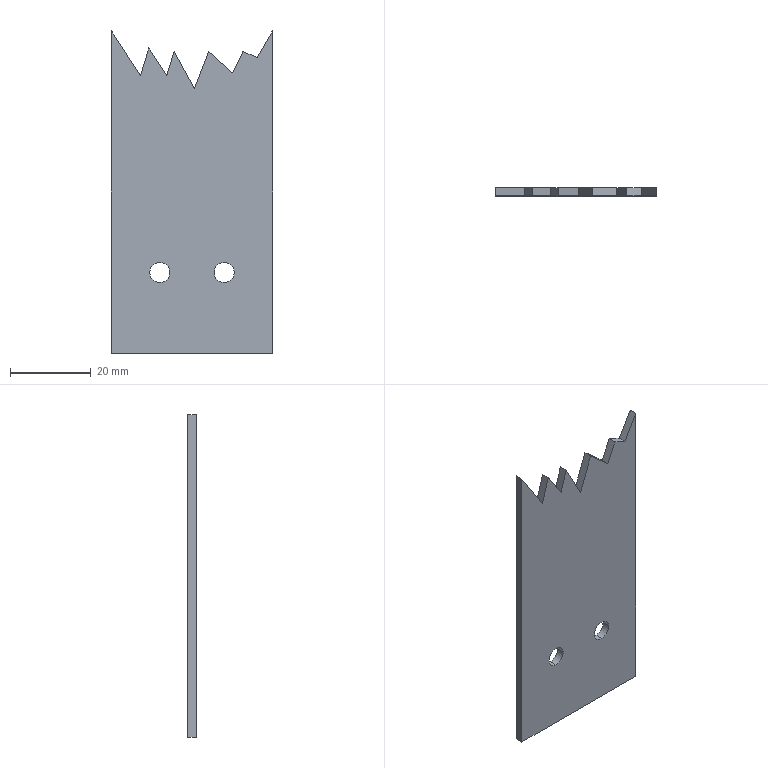Part | SolidWorks | features Cut 2, Extrusion 1 | 1 solid | 19 faces | box 40 x 2 x 80 mm | volume 5747 mm3 | plane 15 | cylinder 4 | commonest cylinder face diameters 5 x4
STEP:
#1=CARTESIAN_POINT('',(8.,2.,-22.5));
#2=VERTEX_POINT('',#1);
#3=CARTESIAN_POINT('',(8.,2.,-17.5));
#4=VERTEX_POINT('',#3);
#5=CARTESIAN_POINT('',(8.,2.,-20.));
#6=DIRECTION('',(0.,1.,0.));
#7=DIRECTION('',(0.,0.,1.));
#8=AXIS2_PLACEMENT_3D('',#5,#6,#7);
#9=CIRCLE('',#8,2.5);
#10=EDGE_CURVE('',#2,#4,#9,.T.);
#11=ORIENTED_EDGE('',*,*,#10,.T.);
#12=CARTESIAN_POINT('',(8.,0.,-17.5));
#13=VERTEX_POINT('',#12);
#14=CARTESIAN_POINT('',(8.,10.,-17.5));
#15=DIRECTION('',(0.,-1.,0.));
#16=VECTOR('',#15,1000.);
#17=LINE('',#14,#16);
#18=EDGE_CURVE('',#4,#13,#17,.T.);
#19=ORIENTED_EDGE('',*,*,#18,.T.);
#20=CARTESIAN_POINT('',(8.,0.,-22.5));
#21=VERTEX_POINT('',#20);
#22=CARTESIAN_POINT('',(8.,0.,-20.));
#23=DIRECTION('',(0.,-1.,0.));
#24=DIRECTION('',(0.,0.,-1.));
#25=AXIS2_PLACEMENT_3D('',#22,#23,#24);
#26=CIRCLE('',#25,2.5);
#27=EDGE_CURVE('',#13,#21,#26,.T.);
#28=ORIENTED_EDGE('',*,*,#27,.T.);
#29=CARTESIAN_POINT('',(8.,10.,-22.5));
#30=DIRECTION('',(0.,-1.,0.));
#31=VECTOR('',#30,1000.);
#32=LINE('',#29,#31);
#33=EDGE_CURVE('',#2,#21,#32,.T.);
#34=ORIENTED_EDGE('',*,*,#33,.F.);
#35=EDGE_LOOP('',(#11,#19,#28,#34));
#36=FACE_OUTER_BOUND('',#35,.T.);
#37=CARTESIAN_POINT('',(8.,10.,-20.));
#38=DIRECTION('',(0.,-1.,0.));
#39=DIRECTION('',(0.,0.,-1.));
#40=AXIS2_PLACEMENT_3D('',#37,#38,#39);
#41=CYLINDRICAL_SURFACE('',#40,2.5);
#42=ADVANCED_FACE('',(#36),#41,.F.);
#43=CARTESIAN_POINT('',(-8.,2.,-22.5));
#44=VERTEX_POINT('',#43);
#45=CARTESIAN_POINT('',(-8.,2.,-17.5));
#46=VERTEX_POINT('',#45);
#47=CARTESIAN_POINT('',(-8.,2.,-20.));
#48=DIRECTION('',(0.,1.,0.));
#49=DIRECTION('',(0.,0.,1.));
#50=AXIS2_PLACEMENT_3D('',#47,#48,#49);
#51=CIRCLE('',#50,2.5);
#52=EDGE_CURVE('',#44,#46,#51,.T.);
#53=ORIENTED_EDGE('',*,*,#52,.T.);
#54=CARTESIAN_POINT('',(-8.,0.,-17.5));
#55=VERTEX_POINT('',#54);
#56=CARTESIAN_POINT('',(-8.,10.,-17.5));
#57=DIRECTION('',(0.,-1.,0.));
#58=VECTOR('',#57,1000.);
#59=LINE('',#56,#58);
#60=EDGE_CURVE('',#46,#55,#59,.T.);
#61=ORIENTED_EDGE('',*,*,#60,.T.);
#62=CARTESIAN_POINT('',(-8.,0.,-22.5));
#63=VERTEX_POINT('',#62);
#64=CARTESIAN_POINT('',(-8.,0.,-20.));
#65=DIRECTION('',(0.,-1.,0.));
#66=DIRECTION('',(0.,0.,-1.));
#67=AXIS2_PLACEMENT_3D('',#64,#65,#66);
#68=CIRCLE('',#67,2.5);
#69=EDGE_CURVE('',#55,#63,#68,.T.);
#70=ORIENTED_EDGE('',*,*,#69,.T.);
#71=CARTESIAN_POINT('',(-8.,10.,-22.5));
#72=DIRECTION('',(0.,-1.,0.));
#73=VECTOR('',#72,1000.);
#74=LINE('',#71,#73);
#75=EDGE_CURVE('',#44,#63,#74,.T.);
#76=ORIENTED_EDGE('',*,*,#75,.F.);
#77=EDGE_LOOP('',(#53,#61,#70,#76));
#78=FACE_OUTER_BOUND('',#77,.T.);
#79=CARTESIAN_POINT('',(-8.,10.,-20.));
#80=DIRECTION('',(0.,-1.,0.));
#81=DIRECTION('',(0.,0.,-1.));
#82=AXIS2_PLACEMENT_3D('',#79,#80,#81);
#83=CYLINDRICAL_SURFACE('',#82,2.5);
#84=ADVANCED_FACE('',(#78),#83,.F.);
#85=CARTESIAN_POINT('',(20.,0.,40.));
#86=VERTEX_POINT('',#85);
#87=CARTESIAN_POINT('',(20.,0.,-40.));
#88=VERTEX_POINT('',#87);
#89=CARTESIAN_POINT('',(20.,0.,-40.));
#90=DIRECTION('',(0.,0.,-1.));
#91=VECTOR('',#90,1000.);
#92=LINE('',#89,#91);
#93=EDGE_CURVE('',#86,#88,#92,.T.);
#94=ORIENTED_EDGE('',*,*,#93,.T.);
#95=CARTESIAN_POINT('',(20.,2.,-40.));
#96=VERTEX_POINT('',#95);
#97=CARTESIAN_POINT('',(20.,2.,-40.));
#98=DIRECTION('',(0.,-1.,0.));
#99=VECTOR('',#98,1000.);
#100=LINE('',#97,#99);
#101=EDGE_CURVE('',#96,#88,#100,.T.);
#102=ORIENTED_EDGE('',*,*,#101,.F.);
#103=CARTESIAN_POINT('',(20.,2.,40.));
#104=VERTEX_POINT('',#103);
#105=CARTESIAN_POINT('',(20.,2.,-40.));
#106=DIRECTION('',(0.,0.,-1.));
#107=VECTOR('',#106,1000.);
#108=LINE('',#105,#107);
#109=EDGE_CURVE('',#104,#96,#108,.T.);
#110=ORIENTED_EDGE('',*,*,#109,.F.);
#111=CARTESIAN_POINT('',(20.,2.,40.));
#112=DIRECTION('',(0.,-1.,0.));
#113=VECTOR('',#112,1000.);
#114=LINE('',#111,#113);
#115=EDGE_CURVE('',#104,#86,#114,.T.);
#116=ORIENTED_EDGE('',*,*,#115,.T.);
#117=EDGE_LOOP('',(#94,#102,#110,#116));
#118=FACE_OUTER_BOUND('',#117,.T.);
#119=CARTESIAN_POINT('',(20.,2.,-40.));
#120=DIRECTION('',(-1.,0.,0.));
#121=DIRECTION('',(0.,0.,1.));
#122=AXIS2_PLACEMENT_3D('',#119,#120,#121);
#123=PLANE('',#122);
#124=ADVANCED_FACE('',(#118),#123,.F.);
#125=CARTESIAN_POINT('',(-20.,0.,-40.));
#126=VERTEX_POINT('',#125);
#127=CARTESIAN_POINT('',(-20.,0.,-40.));
#128=DIRECTION('',(-1.,0.,0.));
#129=VECTOR('',#128,1000.);
#130=LINE('',#127,#129);
#131=EDGE_CURVE('',#88,#126,#130,.T.);
#132=ORIENTED_EDGE('',*,*,#131,.T.);
#133=CARTESIAN_POINT('',(-20.,2.,-40.));
#134=VERTEX_POINT('',#133);
#135=CARTESIAN_POINT('',(-20.,2.,-40.));
#136=DIRECTION('',(0.,-1.,0.));
#137=VECTOR('',#136,1000.);
#138=LINE('',#135,#137);
#139=EDGE_CURVE('',#134,#126,#138,.T.);
#140=ORIENTED_EDGE('',*,*,#139,.F.);
#141=CARTESIAN_POINT('',(-20.,2.,-40.));
#142=DIRECTION('',(-1.,0.,0.));
#143=VECTOR('',#142,1000.);
#144=LINE('',#141,#143);
#145=EDGE_CURVE('',#96,#134,#144,.T.);
#146=ORIENTED_EDGE('',*,*,#145,.F.);
#147=ORIENTED_EDGE('',*,*,#101,.T.);
#148=EDGE_LOOP('',(#132,#140,#146,#147));
#149=FACE_OUTER_BOUND('',#148,.T.);
#150=CARTESIAN_POINT('',(-20.,2.,-40.));
#151=DIRECTION('',(0.,0.,1.));
#152=DIRECTION('',(1.,0.,0.));
#153=AXIS2_PLACEMENT_3D('',#150,#151,#152);
#154=PLANE('',#153);
#155=ADVANCED_FACE('',(#149),#154,.F.);
#156=CARTESIAN_POINT('',(-20.,0.,40.));
#157=VERTEX_POINT('',#156);
#158=CARTESIAN_POINT('',(-20.,0.,-40.));
#159=DIRECTION('',(0.,0.,1.));
#160=VECTOR('',#159,1000.);
#161=LINE('',#158,#160);
#162=EDGE_CURVE('',#126,#157,#161,.T.);
#163=ORIENTED_EDGE('',*,*,#162,.T.);
#164=CARTESIAN_POINT('',(-20.,2.,40.));
#165=VERTEX_POINT('',#164);
#166=CARTESIAN_POINT('',(-20.,2.,40.));
#167=DIRECTION('',(0.,-1.,0.));
#168=VECTOR('',#167,1000.);
#169=LINE('',#166,#168);
#170=EDGE_CURVE('',#165,#157,#169,.T.);
#171=ORIENTED_EDGE('',*,*,#170,.F.);
#172=CARTESIAN_POINT('',(-20.,2.,-40.));
#173=DIRECTION('',(0.,0.,1.));
#174=VECTOR('',#173,1000.);
#175=LINE('',#172,#174);
#176=EDGE_CURVE('',#134,#165,#175,.T.);
#177=ORIENTED_EDGE('',*,*,#176,.F.);
#178=ORIENTED_EDGE('',*,*,#139,.T.);
#179=EDGE_LOOP('',(#163,#171,#177,#178));
#180=FACE_OUTER_BOUND('',#179,.T.);
#181=CARTESIAN_POINT('',(-20.,2.,-40.));
#182=DIRECTION('',(1.,0.,0.));
#183=DIRECTION('',(0.,0.,-1.));
#184=AXIS2_PLACEMENT_3D('',#181,#182,#183);
#185=PLANE('',#184);
#186=ADVANCED_FACE('',(#180),#185,.F.);
#187=CARTESIAN_POINT('',(-12.785,2.,28.891));
#188=VERTEX_POINT('',#187);
#189=CARTESIAN_POINT('',(-20.,2.,40.));
#190=DIRECTION('',(-0.5447,0.,0.8386));
#191=VECTOR('',#190,1000.);
#192=LINE('',#189,#191);
#193=EDGE_CURVE('',#188,#165,#192,.T.);
#194=ORIENTED_EDGE('',*,*,#193,.F.);
#195=CARTESIAN_POINT('',(-10.737,2.,35.779));
#196=VERTEX_POINT('',#195);
#197=CARTESIAN_POINT('',(-12.785,2.,28.891));
#198=DIRECTION('',(-0.285,0.,-0.9585));
#199=VECTOR('',#198,1000.);
#200=LINE('',#197,#199);
#201=EDGE_CURVE('',#196,#188,#200,.T.);
#202=ORIENTED_EDGE('',*,*,#201,.F.);
#203=CARTESIAN_POINT('',(-6.263,2.,28.891));
#204=VERTEX_POINT('',#203);
#205=CARTESIAN_POINT('',(-10.737,2.,35.779));
#206=DIRECTION('',(-0.5447,0.,0.8386));
#207=VECTOR('',#206,1000.);
#208=LINE('',#205,#207);
#209=EDGE_CURVE('',#204,#196,#208,.T.);
#210=ORIENTED_EDGE('',*,*,#209,.F.);
#211=CARTESIAN_POINT('',(-4.459,2.,34.96));
#212=VERTEX_POINT('',#211);
#213=CARTESIAN_POINT('',(-6.263,2.,28.891));
#214=DIRECTION('',(-0.285,0.,-0.9585));
#215=VECTOR('',#214,1000.);
#216=LINE('',#213,#215);
#217=EDGE_CURVE('',#212,#204,#216,.T.);
#218=ORIENTED_EDGE('',*,*,#217,.F.);
#219=CARTESIAN_POINT('',(0.6034,2.,25.613));
#220=VERTEX_POINT('',#219);
#221=CARTESIAN_POINT('',(-4.459,2.,34.96));
#222=DIRECTION('',(-0.4763,0.,0.8793));
#223=VECTOR('',#222,1000.);
#224=LINE('',#221,#223);
#225=EDGE_CURVE('',#220,#212,#224,.T.);
#226=ORIENTED_EDGE('',*,*,#225,.F.);
#227=CARTESIAN_POINT('',(4.155,2.,34.96));
#228=VERTEX_POINT('',#227);
#229=CARTESIAN_POINT('',(0.6034,2.,25.613));
#230=DIRECTION('',(-0.3552,0.,-0.9348));
#231=VECTOR('',#230,1000.);
#232=LINE('',#229,#231);
#233=EDGE_CURVE('',#228,#220,#232,.T.);
#234=ORIENTED_EDGE('',*,*,#233,.F.);
#235=CARTESIAN_POINT('',(10.181,2.,29.56));
#236=VERTEX_POINT('',#235);
#237=CARTESIAN_POINT('',(4.155,2.,34.96));
#238=DIRECTION('',(-0.7448,0.,0.6673));
#239=VECTOR('',#238,1000.);
#240=LINE('',#237,#239);
#241=EDGE_CURVE('',#236,#228,#240,.T.);
#242=ORIENTED_EDGE('',*,*,#241,.F.);
#243=CARTESIAN_POINT('',(12.655,2.,34.96));
#244=VERTEX_POINT('',#243);
#245=CARTESIAN_POINT('',(10.181,2.,29.56));
#246=DIRECTION('',(-0.4166,0.,-0.9091));
#247=VECTOR('',#246,1000.);
#248=LINE('',#245,#247);
#249=EDGE_CURVE('',#244,#236,#248,.T.);
#250=ORIENTED_EDGE('',*,*,#249,.F.);
#251=CARTESIAN_POINT('',(16.161,2.,33.353));
#252=VERTEX_POINT('',#251);
#253=CARTESIAN_POINT('',(12.655,2.,34.96));
#254=DIRECTION('',(-0.9091,0.,0.4166));
#255=VECTOR('',#254,1000.);
#256=LINE('',#253,#255);
#257=EDGE_CURVE('',#252,#244,#256,.T.);
#258=ORIENTED_EDGE('',*,*,#257,.F.);
#259=CARTESIAN_POINT('',(16.161,2.,33.353));
#260=DIRECTION('',(-0.5001,0.,-0.8659));
#261=VECTOR('',#260,1000.);
#262=LINE('',#259,#261);
#263=EDGE_CURVE('',#104,#252,#262,.T.);
#264=ORIENTED_EDGE('',*,*,#263,.F.);
#265=ORIENTED_EDGE('',*,*,#109,.T.);
#266=ORIENTED_EDGE('',*,*,#145,.T.);
#267=ORIENTED_EDGE('',*,*,#176,.T.);
#268=EDGE_LOOP('',(#194,#202,#210,#218,#226,#234,#242,#250,#258,#264,#265,#266,#267));
#269=FACE_OUTER_BOUND('',#268,.T.);
#270=ORIENTED_EDGE('',*,*,#10,.F.);
#271=CARTESIAN_POINT('',(8.,2.,-20.));
#272=DIRECTION('',(0.,1.,0.));
#273=DIRECTION('',(0.,0.,1.));
#274=AXIS2_PLACEMENT_3D('',#271,#272,#273);
#275=CIRCLE('',#274,2.5);
#276=EDGE_CURVE('',#4,#2,#275,.T.);
#277=ORIENTED_EDGE('',*,*,#276,.F.);
#278=EDGE_LOOP('',(#270,#277));
#279=FACE_BOUND('',#278,.T.);
#280=ORIENTED_EDGE('',*,*,#52,.F.);
#281=CARTESIAN_POINT('',(-8.,2.,-20.));
#282=DIRECTION('',(0.,1.,0.));
#283=DIRECTION('',(0.,0.,1.));
#284=AXIS2_PLACEMENT_3D('',#281,#282,#283);
#285=CIRCLE('',#284,2.5);
#286=EDGE_CURVE('',#46,#44,#285,.T.);
#287=ORIENTED_EDGE('',*,*,#286,.F.);
#288=EDGE_LOOP('',(#280,#287));
#289=FACE_BOUND('',#288,.T.);
#290=CARTESIAN_POINT('',(0.,2.,0.));
#291=DIRECTION('',(0.,1.,0.));
#292=DIRECTION('',(0.,0.,1.));
#293=AXIS2_PLACEMENT_3D('',#290,#291,#292);
#294=PLANE('',#293);
#295=ADVANCED_FACE('',(#269,#279,#289),#294,.T.);
#296=CARTESIAN_POINT('',(8.,0.,-20.));
#297=DIRECTION('',(0.,-1.,0.));
#298=DIRECTION('',(0.,0.,-1.));
#299=AXIS2_PLACEMENT_3D('',#296,#297,#298);
#300=CIRCLE('',#299,2.5);
#301=EDGE_CURVE('',#21,#13,#300,.T.);
#302=ORIENTED_EDGE('',*,*,#301,.F.);
#303=ORIENTED_EDGE('',*,*,#27,.F.);
#304=EDGE_LOOP('',(#302,#303));
#305=FACE_BOUND('',#304,.T.);
#306=CARTESIAN_POINT('',(-8.,0.,-20.));
#307=DIRECTION('',(0.,-1.,0.));
#308=DIRECTION('',(0.,0.,-1.));
#309=AXIS2_PLACEMENT_3D('',#306,#307,#308);
#310=CIRCLE('',#309,2.5);
#311=EDGE_CURVE('',#63,#55,#310,.T.);
#312=ORIENTED_EDGE('',*,*,#311,.F.);
#313=ORIENTED_EDGE('',*,*,#69,.F.);
#314=EDGE_LOOP('',(#312,#313));
#315=FACE_BOUND('',#314,.T.);
#316=CARTESIAN_POINT('',(-10.737,0.,35.779));
#317=VERTEX_POINT('',#316);
#318=CARTESIAN_POINT('',(-12.785,0.,28.891));
#319=VERTEX_POINT('',#318);
#320=CARTESIAN_POINT('',(-19.638,0.,5.838));
#321=DIRECTION('',(-0.285,0.,-0.9585));
#322=VECTOR('',#321,1000.);
#323=LINE('',#320,#322);
#324=EDGE_CURVE('',#317,#319,#323,.T.);
#325=ORIENTED_EDGE('',*,*,#324,.T.);
#326=CARTESIAN_POINT('',(4.206,0.,2.732));
#327=DIRECTION('',(-0.5447,0.,0.8386));
#328=VECTOR('',#327,1000.);
#329=LINE('',#326,#328);
#330=EDGE_CURVE('',#319,#157,#329,.T.);
#331=ORIENTED_EDGE('',*,*,#330,.T.);
#332=ORIENTED_EDGE('',*,*,#162,.F.);
#333=ORIENTED_EDGE('',*,*,#131,.F.);
#334=ORIENTED_EDGE('',*,*,#93,.F.);
#335=CARTESIAN_POINT('',(16.161,0.,33.353));
#336=VERTEX_POINT('',#335);
#337=CARTESIAN_POINT('',(-2.326,0.,1.344));
#338=DIRECTION('',(-0.5001,0.,-0.8659));
#339=VECTOR('',#338,1000.);
#340=LINE('',#337,#339);
#341=EDGE_CURVE('',#86,#336,#340,.T.);
#342=ORIENTED_EDGE('',*,*,#341,.T.);
#343=CARTESIAN_POINT('',(12.655,0.,34.96));
#344=VERTEX_POINT('',#343);
#345=CARTESIAN_POINT('',(15.436,0.,33.686));
#346=DIRECTION('',(-0.9091,0.,0.4166));
#347=VECTOR('',#346,1000.);
#348=LINE('',#345,#347);
#349=EDGE_CURVE('',#336,#344,#348,.T.);
#350=ORIENTED_EDGE('',*,*,#349,.T.);
#351=CARTESIAN_POINT('',(10.181,0.,29.56));
#352=VERTEX_POINT('',#351);
#353=CARTESIAN_POINT('',(-2.78,0.,1.274));
#354=DIRECTION('',(-0.4166,0.,-0.9091));
#355=VECTOR('',#354,1000.);
#356=LINE('',#353,#355);
#357=EDGE_CURVE('',#344,#352,#356,.T.);
#358=ORIENTED_EDGE('',*,*,#357,.T.);
#359=CARTESIAN_POINT('',(4.155,0.,34.96));
#360=VERTEX_POINT('',#359);
#361=CARTESIAN_POINT('',(19.225,0.,21.456));
#362=DIRECTION('',(-0.7448,0.,0.6673));
#363=VECTOR('',#362,1000.);
#364=LINE('',#361,#363);
#365=EDGE_CURVE('',#352,#360,#364,.T.);
#366=ORIENTED_EDGE('',*,*,#365,.T.);
#367=CARTESIAN_POINT('',(0.6034,0.,25.613));
#368=VERTEX_POINT('',#367);
#369=CARTESIAN_POINT('',(-7.977,0.,3.031));
#370=DIRECTION('',(-0.3552,0.,-0.9348));
#371=VECTOR('',#370,1000.);
#372=LINE('',#369,#371);
#373=EDGE_CURVE('',#360,#368,#372,.T.);
#374=ORIENTED_EDGE('',*,*,#373,.T.);
#375=CARTESIAN_POINT('',(-4.459,0.,34.96));
#376=VERTEX_POINT('',#375);
#377=CARTESIAN_POINT('',(11.193,0.,6.063));
#378=DIRECTION('',(-0.4763,0.,0.8793));
#379=VECTOR('',#378,1000.);
#380=LINE('',#377,#379);
#381=EDGE_CURVE('',#368,#376,#380,.T.);
#382=ORIENTED_EDGE('',*,*,#381,.T.);
#383=CARTESIAN_POINT('',(-6.263,0.,28.891));
#384=VERTEX_POINT('',#383);
#385=CARTESIAN_POINT('',(-13.647,0.,4.057));
#386=DIRECTION('',(-0.285,0.,-0.9585));
#387=VECTOR('',#386,1000.);
#388=LINE('',#385,#387);
#389=EDGE_CURVE('',#376,#384,#388,.T.);
#390=ORIENTED_EDGE('',*,*,#389,.T.);
#391=CARTESIAN_POINT('',(8.793,0.,5.711));
#392=DIRECTION('',(-0.5447,0.,0.8386));
#393=VECTOR('',#392,1000.);
#394=LINE('',#391,#393);
#395=EDGE_CURVE('',#384,#317,#394,.T.);
#396=ORIENTED_EDGE('',*,*,#395,.T.);
#397=EDGE_LOOP('',(#325,#331,#332,#333,#334,#342,#350,#358,#366,#374,#382,#390,#396));
#398=FACE_OUTER_BOUND('',#397,.T.);
#399=CARTESIAN_POINT('',(0.,0.,0.));
#400=DIRECTION('',(0.,1.,0.));
#401=DIRECTION('',(0.,0.,1.));
#402=AXIS2_PLACEMENT_3D('',#399,#400,#401);
#403=PLANE('',#402);
#404=ADVANCED_FACE('',(#305,#315,#398),#403,.F.);
#405=ORIENTED_EDGE('',*,*,#60,.F.);
#406=ORIENTED_EDGE('',*,*,#286,.T.);
#407=ORIENTED_EDGE('',*,*,#75,.T.);
#408=ORIENTED_EDGE('',*,*,#311,.T.);
#409=EDGE_LOOP('',(#405,#406,#407,#408));
#410=FACE_OUTER_BOUND('',#409,.T.);
#411=CARTESIAN_POINT('',(-8.,10.,-20.));
#412=DIRECTION('',(0.,-1.,0.));
#413=DIRECTION('',(0.,0.,-1.));
#414=AXIS2_PLACEMENT_3D('',#411,#412,#413);
#415=CYLINDRICAL_SURFACE('',#414,2.5);
#416=ADVANCED_FACE('',(#410),#415,.F.);
#417=ORIENTED_EDGE('',*,*,#18,.F.);
#418=ORIENTED_EDGE('',*,*,#276,.T.);
#419=ORIENTED_EDGE('',*,*,#33,.T.);
#420=ORIENTED_EDGE('',*,*,#301,.T.);
#421=EDGE_LOOP('',(#417,#418,#419,#420));
#422=FACE_OUTER_BOUND('',#421,.T.);
#423=CARTESIAN_POINT('',(8.,10.,-20.));
#424=DIRECTION('',(0.,-1.,0.));
#425=DIRECTION('',(0.,0.,-1.));
#426=AXIS2_PLACEMENT_3D('',#423,#424,#425);
#427=CYLINDRICAL_SURFACE('',#426,2.5);
#428=ADVANCED_FACE('',(#422),#427,.F.);
#429=CARTESIAN_POINT('',(-12.785,-8.,28.891));
#430=DIRECTION('',(0.,1.,0.));
#431=VECTOR('',#430,1000.);
#432=LINE('',#429,#431);
#433=EDGE_CURVE('',#319,#188,#432,.T.);
#434=ORIENTED_EDGE('',*,*,#433,.T.);
#435=ORIENTED_EDGE('',*,*,#193,.T.);
#436=ORIENTED_EDGE('',*,*,#170,.T.);
#437=ORIENTED_EDGE('',*,*,#330,.F.);
#438=EDGE_LOOP('',(#434,#435,#436,#437));
#439=FACE_OUTER_BOUND('',#438,.T.);
#440=CARTESIAN_POINT('',(-20.,-8.,40.));
#441=DIRECTION('',(-0.8386,0.,-0.5447));
#442=DIRECTION('',(-0.5447,0.,0.8386));
#443=AXIS2_PLACEMENT_3D('',#440,#441,#442);
#444=PLANE('',#443);
#445=ADVANCED_FACE('',(#439),#444,.F.);
#446=CARTESIAN_POINT('',(-10.737,-8.,35.779));
#447=DIRECTION('',(0.,1.,0.));
#448=VECTOR('',#447,1000.);
#449=LINE('',#446,#448);
#450=EDGE_CURVE('',#317,#196,#449,.T.);
#451=ORIENTED_EDGE('',*,*,#450,.T.);
#452=ORIENTED_EDGE('',*,*,#201,.T.);
#453=ORIENTED_EDGE('',*,*,#433,.F.);
#454=ORIENTED_EDGE('',*,*,#324,.F.);
#455=EDGE_LOOP('',(#451,#452,#453,#454));
#456=FACE_OUTER_BOUND('',#455,.T.);
#457=CARTESIAN_POINT('',(-12.785,-8.,28.891));
#458=DIRECTION('',(0.9585,0.,-0.285));
#459=DIRECTION('',(-0.285,0.,-0.9585));
#460=AXIS2_PLACEMENT_3D('',#457,#458,#459);
#461=PLANE('',#460);
#462=ADVANCED_FACE('',(#456),#461,.F.);
#463=CARTESIAN_POINT('',(-6.263,-8.,28.891));
#464=DIRECTION('',(0.,1.,0.));
#465=VECTOR('',#464,1000.);
#466=LINE('',#463,#465);
#467=EDGE_CURVE('',#384,#204,#466,.T.);
#468=ORIENTED_EDGE('',*,*,#467,.T.);
#469=ORIENTED_EDGE('',*,*,#209,.T.);
#470=ORIENTED_EDGE('',*,*,#450,.F.);
#471=ORIENTED_EDGE('',*,*,#395,.F.);
#472=EDGE_LOOP('',(#468,#469,#470,#471));
#473=FACE_OUTER_BOUND('',#472,.T.);
#474=CARTESIAN_POINT('',(-10.737,-8.,35.779));
#475=DIRECTION('',(-0.8386,0.,-0.5447));
#476=DIRECTION('',(-0.5447,0.,0.8386));
#477=AXIS2_PLACEMENT_3D('',#474,#475,#476);
#478=PLANE('',#477);
#479=ADVANCED_FACE('',(#473),#478,.F.);
#480=CARTESIAN_POINT('',(-4.459,-8.,34.96));
#481=DIRECTION('',(0.,1.,0.));
#482=VECTOR('',#481,1000.);
#483=LINE('',#480,#482);
#484=EDGE_CURVE('',#376,#212,#483,.T.);
#485=ORIENTED_EDGE('',*,*,#484,.T.);
#486=ORIENTED_EDGE('',*,*,#217,.T.);
#487=ORIENTED_EDGE('',*,*,#467,.F.);
#488=ORIENTED_EDGE('',*,*,#389,.F.);
#489=EDGE_LOOP('',(#485,#486,#487,#488));
#490=FACE_OUTER_BOUND('',#489,.T.);
#491=CARTESIAN_POINT('',(-6.263,-8.,28.891));
#492=DIRECTION('',(0.9585,0.,-0.285));
#493=DIRECTION('',(-0.285,0.,-0.9585));
#494=AXIS2_PLACEMENT_3D('',#491,#492,#493);
#495=PLANE('',#494);
#496=ADVANCED_FACE('',(#490),#495,.F.);
#497=CARTESIAN_POINT('',(0.6034,-8.,25.613));
#498=DIRECTION('',(0.,1.,0.));
#499=VECTOR('',#498,1000.);
#500=LINE('',#497,#499);
#501=EDGE_CURVE('',#368,#220,#500,.T.);
#502=ORIENTED_EDGE('',*,*,#501,.T.);
#503=ORIENTED_EDGE('',*,*,#225,.T.);
#504=ORIENTED_EDGE('',*,*,#484,.F.);
#505=ORIENTED_EDGE('',*,*,#381,.F.);
#506=EDGE_LOOP('',(#502,#503,#504,#505));
#507=FACE_OUTER_BOUND('',#506,.T.);
#508=CARTESIAN_POINT('',(-4.459,-8.,34.96));
#509=DIRECTION('',(-0.8793,0.,-0.4763));
#510=DIRECTION('',(-0.4763,0.,0.8793));
#511=AXIS2_PLACEMENT_3D('',#508,#509,#510);
#512=PLANE('',#511);
#513=ADVANCED_FACE('',(#507),#512,.F.);
#514=CARTESIAN_POINT('',(4.155,-8.,34.96));
#515=DIRECTION('',(0.,1.,0.));
#516=VECTOR('',#515,1000.);
#517=LINE('',#514,#516);
#518=EDGE_CURVE('',#360,#228,#517,.T.);
#519=ORIENTED_EDGE('',*,*,#518,.T.);
#520=ORIENTED_EDGE('',*,*,#233,.T.);
#521=ORIENTED_EDGE('',*,*,#501,.F.);
#522=ORIENTED_EDGE('',*,*,#373,.F.);
#523=EDGE_LOOP('',(#519,#520,#521,#522));
#524=FACE_OUTER_BOUND('',#523,.T.);
#525=CARTESIAN_POINT('',(0.6034,-8.,25.613));
#526=DIRECTION('',(0.9348,0.,-0.3552));
#527=DIRECTION('',(-0.3552,0.,-0.9348));
#528=AXIS2_PLACEMENT_3D('',#525,#526,#527);
#529=PLANE('',#528);
#530=ADVANCED_FACE('',(#524),#529,.F.);
#531=CARTESIAN_POINT('',(10.181,-8.,29.56));
#532=DIRECTION('',(0.,1.,0.));
#533=VECTOR('',#532,1000.);
#534=LINE('',#531,#533);
#535=EDGE_CURVE('',#352,#236,#534,.T.);
#536=ORIENTED_EDGE('',*,*,#535,.T.);
#537=ORIENTED_EDGE('',*,*,#241,.T.);
#538=ORIENTED_EDGE('',*,*,#518,.F.);
#539=ORIENTED_EDGE('',*,*,#365,.F.);
#540=EDGE_LOOP('',(#536,#537,#538,#539));
#541=FACE_OUTER_BOUND('',#540,.T.);
#542=CARTESIAN_POINT('',(4.155,-8.,34.96));
#543=DIRECTION('',(-0.6673,0.,-0.7448));
#544=DIRECTION('',(-0.7448,0.,0.6673));
#545=AXIS2_PLACEMENT_3D('',#542,#543,#544);
#546=PLANE('',#545);
#547=ADVANCED_FACE('',(#541),#546,.F.);
#548=CARTESIAN_POINT('',(12.655,-8.,34.96));
#549=DIRECTION('',(0.,1.,0.));
#550=VECTOR('',#549,1000.);
#551=LINE('',#548,#550);
#552=EDGE_CURVE('',#344,#244,#551,.T.);
#553=ORIENTED_EDGE('',*,*,#552,.T.);
#554=ORIENTED_EDGE('',*,*,#249,.T.);
#555=ORIENTED_EDGE('',*,*,#535,.F.);
#556=ORIENTED_EDGE('',*,*,#357,.F.);
#557=EDGE_LOOP('',(#553,#554,#555,#556));
#558=FACE_OUTER_BOUND('',#557,.T.);
#559=CARTESIAN_POINT('',(10.181,-8.,29.56));
#560=DIRECTION('',(0.9091,0.,-0.4166));
#561=DIRECTION('',(-0.4166,0.,-0.9091));
#562=AXIS2_PLACEMENT_3D('',#559,#560,#561);
#563=PLANE('',#562);
#564=ADVANCED_FACE('',(#558),#563,.F.);
#565=CARTESIAN_POINT('',(16.161,-8.,33.353));
#566=DIRECTION('',(0.,1.,0.));
#567=VECTOR('',#566,1000.);
#568=LINE('',#565,#567);
#569=EDGE_CURVE('',#336,#252,#568,.T.);
#570=ORIENTED_EDGE('',*,*,#569,.T.);
#571=ORIENTED_EDGE('',*,*,#257,.T.);
#572=ORIENTED_EDGE('',*,*,#552,.F.);
#573=ORIENTED_EDGE('',*,*,#349,.F.);
#574=EDGE_LOOP('',(#570,#571,#572,#573));
#575=FACE_OUTER_BOUND('',#574,.T.);
#576=CARTESIAN_POINT('',(12.655,-8.,34.96));
#577=DIRECTION('',(-0.4166,0.,-0.9091));
#578=DIRECTION('',(-0.9091,0.,0.4166));
#579=AXIS2_PLACEMENT_3D('',#576,#577,#578);
#580=PLANE('',#579);
#581=ADVANCED_FACE('',(#575),#580,.F.);
#582=ORIENTED_EDGE('',*,*,#115,.F.);
#583=ORIENTED_EDGE('',*,*,#263,.T.);
#584=ORIENTED_EDGE('',*,*,#569,.F.);
#585=ORIENTED_EDGE('',*,*,#341,.F.);
#586=EDGE_LOOP('',(#582,#583,#584,#585));
#587=FACE_OUTER_BOUND('',#586,.T.);
#588=CARTESIAN_POINT('',(16.161,-8.,33.353));
#589=DIRECTION('',(0.8659,0.,-0.5001));
#590=DIRECTION('',(-0.5001,0.,-0.8659));
#591=AXIS2_PLACEMENT_3D('',#588,#589,#590);
#592=PLANE('',#591);
#593=ADVANCED_FACE('',(#587),#592,.F.);
#594=CLOSED_SHELL('',(#42,#84,#124,#155,#186,#295,#404,#416,#428,#445,#462,#479,#496,#513,#530,#547,#564,#581,#593));
#595=MANIFOLD_SOLID_BREP('',#594);
#596=CARTESIAN_POINT('',(0.,0.,0.));
#597=DIRECTION('',(0.,0.,1.));
#598=DIRECTION('',(1.,0.,0.));
#599=AXIS2_PLACEMENT_3D('',#596,#597,#598);
#600=(LENGTH_UNIT()NAMED_UNIT(*)SI_UNIT(.MILLI.,.METRE.));
#601=UNCERTAINTY_MEASURE_WITH_UNIT(LENGTH_MEASURE(0.00001),#600,'','');
#602=(NAMED_UNIT(*)PLANE_ANGLE_UNIT()SI_UNIT($,.RADIAN.));
#603=(NAMED_UNIT(*)SI_UNIT($,.STERADIAN.)SOLID_ANGLE_UNIT());
#604=(GEOMETRIC_REPRESENTATION_CONTEXT(3)GLOBAL_UNCERTAINTY_ASSIGNED_CONTEXT((#601))GLOBAL_UNIT_ASSIGNED_CONTEXT((#600,#602,#603))REPRESENTATION_CONTEXT('',''));
#605=ADVANCED_BREP_SHAPE_REPRESENTATION('',(#595,#599),#604);